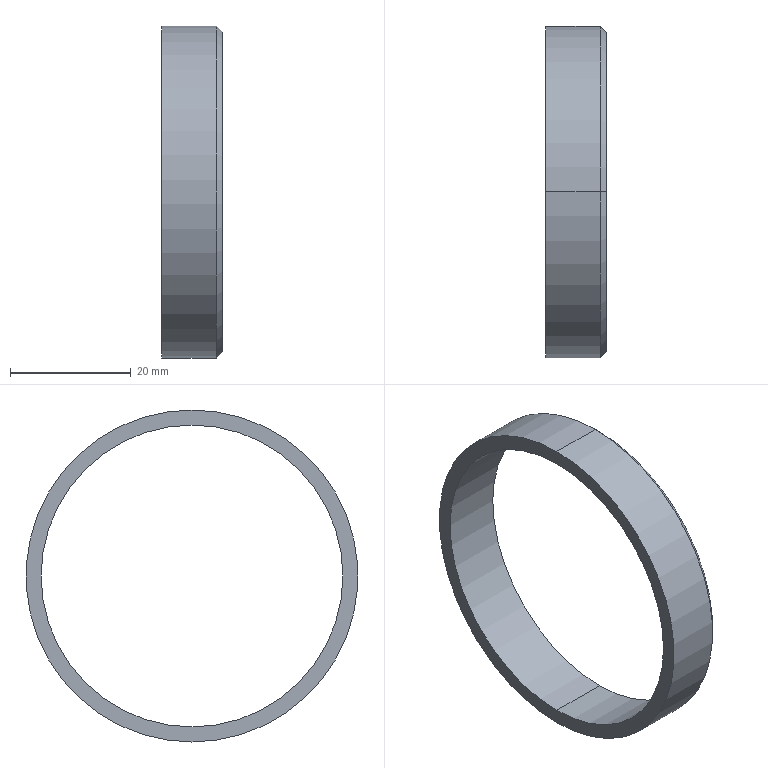Part | SolidWorks | features Chamfer 1, Revolution 1 | 1 solid | 8 faces | box 10 x 55 x 55 mm | volume 4038 mm3 | cylinder 4 | cone 2 | plane 2 | commonest cylinder face diameters 50 x2 55 x2
STEP:
#1=CARTESIAN_POINT('',(10.,0.,-26.5));
#2=VERTEX_POINT('',#1);
#3=CARTESIAN_POINT('',(10.,0.,26.5));
#4=VERTEX_POINT('',#3);
#5=CARTESIAN_POINT('',(10.,0.,0.));
#6=DIRECTION('',(1.,0.,0.));
#7=DIRECTION('',(0.,0.,1.));
#8=AXIS2_PLACEMENT_3D('',#5,#6,#7);
#9=CIRCLE('',#8,26.5);
#10=EDGE_CURVE('',#2,#4,#9,.T.);
#11=ORIENTED_EDGE('',*,*,#10,.F.);
#12=CARTESIAN_POINT('',(9.,0.,-27.5));
#13=VERTEX_POINT('',#12);
#14=CARTESIAN_POINT('',(9.,0.,-27.5));
#15=DIRECTION('',(-0.7071,0.,-0.7071));
#16=VECTOR('',#15,1000.);
#17=LINE('',#14,#16);
#18=EDGE_CURVE('',#2,#13,#17,.T.);
#19=ORIENTED_EDGE('',*,*,#18,.T.);
#20=CARTESIAN_POINT('',(9.,0.,27.5));
#21=VERTEX_POINT('',#20);
#22=CARTESIAN_POINT('',(9.,0.,0.));
#23=DIRECTION('',(-1.,0.,0.));
#24=DIRECTION('',(0.,0.,1.));
#25=AXIS2_PLACEMENT_3D('',#22,#23,#24);
#26=CIRCLE('',#25,27.5);
#27=EDGE_CURVE('',#21,#13,#26,.T.);
#28=ORIENTED_EDGE('',*,*,#27,.F.);
#29=CARTESIAN_POINT('',(9.,0.,27.5));
#30=DIRECTION('',(-0.7071,0.,0.7071));
#31=VECTOR('',#30,1000.);
#32=LINE('',#29,#31);
#33=EDGE_CURVE('',#4,#21,#32,.T.);
#34=ORIENTED_EDGE('',*,*,#33,.F.);
#35=EDGE_LOOP('',(#11,#19,#28,#34));
#36=FACE_OUTER_BOUND('',#35,.T.);
#37=CARTESIAN_POINT('',(9.,0.,0.));
#38=DIRECTION('',(-1.,0.,0.));
#39=DIRECTION('',(0.,0.,1.));
#40=AXIS2_PLACEMENT_3D('',#37,#38,#39);
#41=CONICAL_SURFACE('',#40,27.5,0.7854);
#42=ADVANCED_FACE('',(#36),#41,.T.);
#43=ORIENTED_EDGE('',*,*,#27,.T.);
#44=CARTESIAN_POINT('',(0.,0.,-27.5));
#45=VERTEX_POINT('',#44);
#46=CARTESIAN_POINT('',(-308.213,0.,-27.5));
#47=DIRECTION('',(-1.,0.,0.));
#48=VECTOR('',#47,1000.);
#49=LINE('',#46,#48);
#50=EDGE_CURVE('',#13,#45,#49,.T.);
#51=ORIENTED_EDGE('',*,*,#50,.T.);
#52=CARTESIAN_POINT('',(0.,0.,27.5));
#53=VERTEX_POINT('',#52);
#54=CARTESIAN_POINT('',(0.,0.,0.));
#55=DIRECTION('',(-1.,0.,0.));
#56=DIRECTION('',(0.,0.,1.));
#57=AXIS2_PLACEMENT_3D('',#54,#55,#56);
#58=CIRCLE('',#57,27.5);
#59=EDGE_CURVE('',#53,#45,#58,.T.);
#60=ORIENTED_EDGE('',*,*,#59,.F.);
#61=CARTESIAN_POINT('',(-308.213,0.,27.5));
#62=DIRECTION('',(-1.,0.,0.));
#63=VECTOR('',#62,1000.);
#64=LINE('',#61,#63);
#65=EDGE_CURVE('',#21,#53,#64,.T.);
#66=ORIENTED_EDGE('',*,*,#65,.F.);
#67=EDGE_LOOP('',(#43,#51,#60,#66));
#68=FACE_OUTER_BOUND('',#67,.T.);
#69=CARTESIAN_POINT('',(-308.213,0.,0.));
#70=DIRECTION('',(-1.,0.,0.));
#71=DIRECTION('',(0.,0.,1.));
#72=AXIS2_PLACEMENT_3D('',#69,#70,#71);
#73=CYLINDRICAL_SURFACE('',#72,27.5);
#74=ADVANCED_FACE('',(#68),#73,.T.);
#75=CARTESIAN_POINT('',(10.,0.,-25.));
#76=VERTEX_POINT('',#75);
#77=CARTESIAN_POINT('',(10.,0.,25.));
#78=VERTEX_POINT('',#77);
#79=CARTESIAN_POINT('',(10.,0.,0.));
#80=DIRECTION('',(-1.,0.,0.));
#81=DIRECTION('',(0.,0.,1.));
#82=AXIS2_PLACEMENT_3D('',#79,#80,#81);
#83=CIRCLE('',#82,25.);
#84=EDGE_CURVE('',#76,#78,#83,.T.);
#85=ORIENTED_EDGE('',*,*,#84,.F.);
#86=CARTESIAN_POINT('',(0.,0.,-25.));
#87=VERTEX_POINT('',#86);
#88=CARTESIAN_POINT('',(-308.213,0.,-25.));
#89=DIRECTION('',(-1.,0.,0.));
#90=VECTOR('',#89,1000.);
#91=LINE('',#88,#90);
#92=EDGE_CURVE('',#76,#87,#91,.T.);
#93=ORIENTED_EDGE('',*,*,#92,.T.);
#94=CARTESIAN_POINT('',(0.,0.,25.));
#95=VERTEX_POINT('',#94);
#96=CARTESIAN_POINT('',(0.,0.,0.));
#97=DIRECTION('',(-1.,0.,0.));
#98=DIRECTION('',(0.,0.,1.));
#99=AXIS2_PLACEMENT_3D('',#96,#97,#98);
#100=CIRCLE('',#99,25.);
#101=EDGE_CURVE('',#87,#95,#100,.T.);
#102=ORIENTED_EDGE('',*,*,#101,.T.);
#103=CARTESIAN_POINT('',(-308.213,0.,25.));
#104=DIRECTION('',(-1.,0.,0.));
#105=VECTOR('',#104,1000.);
#106=LINE('',#103,#105);
#107=EDGE_CURVE('',#78,#95,#106,.T.);
#108=ORIENTED_EDGE('',*,*,#107,.F.);
#109=EDGE_LOOP('',(#85,#93,#102,#108));
#110=FACE_OUTER_BOUND('',#109,.T.);
#111=CARTESIAN_POINT('',(-308.213,0.,0.));
#112=DIRECTION('',(-1.,0.,0.));
#113=DIRECTION('',(0.,0.,1.));
#114=AXIS2_PLACEMENT_3D('',#111,#112,#113);
#115=CYLINDRICAL_SURFACE('',#114,25.);
#116=ADVANCED_FACE('',(#110),#115,.F.);
#117=ORIENTED_EDGE('',*,*,#92,.F.);
#118=CARTESIAN_POINT('',(10.,0.,0.));
#119=DIRECTION('',(-1.,0.,0.));
#120=DIRECTION('',(0.,0.,1.));
#121=AXIS2_PLACEMENT_3D('',#118,#119,#120);
#122=CIRCLE('',#121,25.);
#123=EDGE_CURVE('',#78,#76,#122,.T.);
#124=ORIENTED_EDGE('',*,*,#123,.F.);
#125=ORIENTED_EDGE('',*,*,#107,.T.);
#126=CARTESIAN_POINT('',(0.,0.,0.));
#127=DIRECTION('',(-1.,0.,0.));
#128=DIRECTION('',(0.,0.,1.));
#129=AXIS2_PLACEMENT_3D('',#126,#127,#128);
#130=CIRCLE('',#129,25.);
#131=EDGE_CURVE('',#95,#87,#130,.T.);
#132=ORIENTED_EDGE('',*,*,#131,.T.);
#133=EDGE_LOOP('',(#117,#124,#125,#132));
#134=FACE_OUTER_BOUND('',#133,.T.);
#135=CARTESIAN_POINT('',(-308.213,0.,0.));
#136=DIRECTION('',(-1.,0.,0.));
#137=DIRECTION('',(0.,0.,1.));
#138=AXIS2_PLACEMENT_3D('',#135,#136,#137);
#139=CYLINDRICAL_SURFACE('',#138,25.);
#140=ADVANCED_FACE('',(#134),#139,.F.);
#141=ORIENTED_EDGE('',*,*,#131,.F.);
#142=ORIENTED_EDGE('',*,*,#101,.F.);
#143=EDGE_LOOP('',(#141,#142));
#144=FACE_BOUND('',#143,.T.);
#145=ORIENTED_EDGE('',*,*,#59,.T.);
#146=CARTESIAN_POINT('',(0.,0.,0.));
#147=DIRECTION('',(-1.,0.,0.));
#148=DIRECTION('',(0.,0.,1.));
#149=AXIS2_PLACEMENT_3D('',#146,#147,#148);
#150=CIRCLE('',#149,27.5);
#151=EDGE_CURVE('',#45,#53,#150,.T.);
#152=ORIENTED_EDGE('',*,*,#151,.T.);
#153=EDGE_LOOP('',(#145,#152));
#154=FACE_OUTER_BOUND('',#153,.T.);
#155=CARTESIAN_POINT('',(0.,0.,-25.));
#156=DIRECTION('',(1.,0.,0.));
#157=DIRECTION('',(0.,0.,-1.));
#158=AXIS2_PLACEMENT_3D('',#155,#156,#157);
#159=PLANE('',#158);
#160=ADVANCED_FACE('',(#144,#154),#159,.F.);
#161=ORIENTED_EDGE('',*,*,#50,.F.);
#162=CARTESIAN_POINT('',(9.,0.,0.));
#163=DIRECTION('',(-1.,0.,0.));
#164=DIRECTION('',(0.,0.,1.));
#165=AXIS2_PLACEMENT_3D('',#162,#163,#164);
#166=CIRCLE('',#165,27.5);
#167=EDGE_CURVE('',#13,#21,#166,.T.);
#168=ORIENTED_EDGE('',*,*,#167,.T.);
#169=ORIENTED_EDGE('',*,*,#65,.T.);
#170=ORIENTED_EDGE('',*,*,#151,.F.);
#171=EDGE_LOOP('',(#161,#168,#169,#170));
#172=FACE_OUTER_BOUND('',#171,.T.);
#173=CARTESIAN_POINT('',(-308.213,0.,0.));
#174=DIRECTION('',(-1.,0.,0.));
#175=DIRECTION('',(0.,0.,1.));
#176=AXIS2_PLACEMENT_3D('',#173,#174,#175);
#177=CYLINDRICAL_SURFACE('',#176,27.5);
#178=ADVANCED_FACE('',(#172),#177,.T.);
#179=CARTESIAN_POINT('',(10.,0.,0.));
#180=DIRECTION('',(1.,0.,0.));
#181=DIRECTION('',(0.,0.,1.));
#182=AXIS2_PLACEMENT_3D('',#179,#180,#181);
#183=CIRCLE('',#182,26.5);
#184=EDGE_CURVE('',#4,#2,#183,.T.);
#185=ORIENTED_EDGE('',*,*,#184,.T.);
#186=ORIENTED_EDGE('',*,*,#10,.T.);
#187=EDGE_LOOP('',(#185,#186));
#188=FACE_OUTER_BOUND('',#187,.T.);
#189=ORIENTED_EDGE('',*,*,#123,.T.);
#190=ORIENTED_EDGE('',*,*,#84,.T.);
#191=EDGE_LOOP('',(#189,#190));
#192=FACE_BOUND('',#191,.T.);
#193=CARTESIAN_POINT('',(10.,0.,-27.5));
#194=DIRECTION('',(-1.,0.,0.));
#195=DIRECTION('',(0.,0.,1.));
#196=AXIS2_PLACEMENT_3D('',#193,#194,#195);
#197=PLANE('',#196);
#198=ADVANCED_FACE('',(#188,#192),#197,.F.);
#199=ORIENTED_EDGE('',*,*,#18,.F.);
#200=ORIENTED_EDGE('',*,*,#184,.F.);
#201=ORIENTED_EDGE('',*,*,#33,.T.);
#202=ORIENTED_EDGE('',*,*,#167,.F.);
#203=EDGE_LOOP('',(#199,#200,#201,#202));
#204=FACE_OUTER_BOUND('',#203,.T.);
#205=CARTESIAN_POINT('',(9.,0.,0.));
#206=DIRECTION('',(-1.,0.,0.));
#207=DIRECTION('',(0.,0.,1.));
#208=AXIS2_PLACEMENT_3D('',#205,#206,#207);
#209=CONICAL_SURFACE('',#208,27.5,0.7854);
#210=ADVANCED_FACE('',(#204),#209,.T.);
#211=CLOSED_SHELL('',(#42,#74,#116,#140,#160,#178,#198,#210));
#212=MANIFOLD_SOLID_BREP('',#211);
#213=CARTESIAN_POINT('',(0.,0.,0.));
#214=DIRECTION('',(0.,0.,1.));
#215=DIRECTION('',(1.,0.,0.));
#216=AXIS2_PLACEMENT_3D('',#213,#214,#215);
#217=(LENGTH_UNIT()NAMED_UNIT(*)SI_UNIT(.MILLI.,.METRE.));
#218=UNCERTAINTY_MEASURE_WITH_UNIT(LENGTH_MEASURE(0.00001),#217,'','');
#219=(NAMED_UNIT(*)PLANE_ANGLE_UNIT()SI_UNIT($,.RADIAN.));
#220=(NAMED_UNIT(*)SI_UNIT($,.STERADIAN.)SOLID_ANGLE_UNIT());
#221=(GEOMETRIC_REPRESENTATION_CONTEXT(3)GLOBAL_UNCERTAINTY_ASSIGNED_CONTEXT((#218))GLOBAL_UNIT_ASSIGNED_CONTEXT((#217,#219,#220))REPRESENTATION_CONTEXT('',''));
#222=ADVANCED_BREP_SHAPE_REPRESENTATION('',(#212,#216),#221);